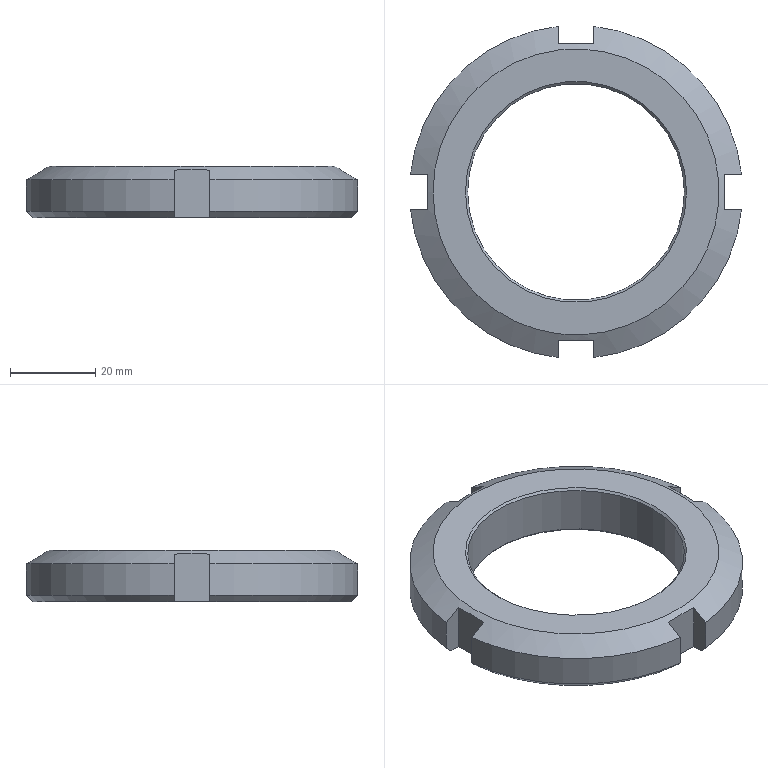Part | NX | features INSTANCE 4, CHAMFER 2, DATUM_CSYS 2, SKETCH 2, CIRCULAR_ISET 1, EXTRUDE 1, FSET 1, LINE 1, META 1, SWP104 1, SYMBOLIC_THREAD 1, THREADS 1, TRANSFORM_ISET 1 | 1 solid | 26 faces | box 77.551 x 77.551 x 12 mm | volume 29319 mm3 | plane 14 | cone 7 | cylinder 5 | commonest cylinder face diameters 78 x4 50.782 x1
STEP:
#1=CARTESIAN_POINT('',(-38.775,-4.18,1.5));
#2=VERTEX_POINT('',#1);
#3=CARTESIAN_POINT('',(-4.18,-38.775,1.5));
#4=VERTEX_POINT('',#3);
#5=CARTESIAN_POINT('',(0.,0.,1.5));
#6=DIRECTION('',(0.,0.,1.));
#7=DIRECTION('',(1.,0.,0.));
#8=AXIS2_PLACEMENT_3D('',#5,#6,#7);
#9=CIRCLE('',#8,39.);
#10=EDGE_CURVE('',#2,#4,#9,.T.);
#11=ORIENTED_EDGE('',*,*,#10,.T.);
#12=CARTESIAN_POINT('',(-4.18,-38.775,8.825));
#13=VERTEX_POINT('',#12);
#14=CARTESIAN_POINT('',(-4.18,-38.775,0.));
#15=DIRECTION('',(0.,0.,-1.));
#16=VECTOR('',#15,1000.);
#17=LINE('',#14,#16);
#18=EDGE_CURVE('',#4,#13,#17,.F.);
#19=ORIENTED_EDGE('',*,*,#18,.T.);
#20=CARTESIAN_POINT('',(-38.775,-4.18,8.825));
#21=VERTEX_POINT('',#20);
#22=CARTESIAN_POINT('',(0.,0.,8.825));
#23=DIRECTION('',(0.,0.,-1.));
#24=DIRECTION('',(-1.,0.,0.));
#25=AXIS2_PLACEMENT_3D('',#22,#23,#24);
#26=CIRCLE('',#25,39.);
#27=EDGE_CURVE('',#13,#21,#26,.T.);
#28=ORIENTED_EDGE('',*,*,#27,.T.);
#29=CARTESIAN_POINT('',(-38.775,-4.18,0.));
#30=DIRECTION('',(0.,0.,-1.));
#31=VECTOR('',#30,1000.);
#32=LINE('',#29,#31);
#33=EDGE_CURVE('',#21,#2,#32,.T.);
#34=ORIENTED_EDGE('',*,*,#33,.T.);
#35=EDGE_LOOP('',(#11,#19,#28,#34));
#36=FACE_BOUND('',#35,.T.);
#37=CARTESIAN_POINT('',(0.,0.,0.));
#38=DIRECTION('',(0.,0.,-1.));
#39=DIRECTION('',(-1.,0.,0.));
#40=AXIS2_PLACEMENT_3D('',#37,#38,#39);
#41=CYLINDRICAL_SURFACE('',#40,39.);
#42=ADVANCED_FACE('',(#36),#41,.T.);
#43=CARTESIAN_POINT('',(-4.18,-37.266,0.));
#44=VERTEX_POINT('',#43);
#45=CARTESIAN_POINT('',(-4.18,-38.775,1.5));
#46=CARTESIAN_POINT('',(-4.18,-38.272,0.9999));
#47=CARTESIAN_POINT('',(-4.18,-37.769,0.4999));
#48=CARTESIAN_POINT('',(-4.18,-37.266,0.));
#49=B_SPLINE_CURVE_WITH_KNOTS('',3,(#45,#46,#47,#48),.UNSPECIFIED.,.F.,.F.,(4,4),(0.008129,0.01026),.UNSPECIFIED.);
#50=EDGE_CURVE('',#4,#44,#49,.T.);
#51=ORIENTED_EDGE('',*,*,#50,.F.);
#52=ORIENTED_EDGE('',*,*,#10,.F.);
#53=CARTESIAN_POINT('',(-37.266,-4.18,0.));
#54=VERTEX_POINT('',#53);
#55=CARTESIAN_POINT('',(-37.266,-4.18,0.));
#56=CARTESIAN_POINT('',(-37.769,-4.18,0.4999));
#57=CARTESIAN_POINT('',(-38.272,-4.18,0.9999));
#58=CARTESIAN_POINT('',(-38.775,-4.18,1.5));
#59=B_SPLINE_CURVE_WITH_KNOTS('',3,(#55,#56,#57,#58),.UNSPECIFIED.,.F.,.F.,(4,4),(0.007494,0.009622),.UNSPECIFIED.);
#60=EDGE_CURVE('',#54,#2,#59,.T.);
#61=ORIENTED_EDGE('',*,*,#60,.F.);
#62=CARTESIAN_POINT('',(0.,0.,0.));
#63=DIRECTION('',(0.,0.,1.));
#64=DIRECTION('',(1.,0.,0.));
#65=AXIS2_PLACEMENT_3D('',#62,#63,#64);
#66=CIRCLE('',#65,37.5);
#67=EDGE_CURVE('',#44,#54,#66,.F.);
#68=ORIENTED_EDGE('',*,*,#67,.F.);
#69=EDGE_LOOP('',(#51,#52,#61,#68));
#70=FACE_BOUND('',#69,.T.);
#71=CARTESIAN_POINT('',(0.,0.,0.));
#72=DIRECTION('',(0.,0.,1.));
#73=DIRECTION('',(1.,0.,0.));
#74=AXIS2_PLACEMENT_3D('',#71,#72,#73);
#75=CONICAL_SURFACE('',#74,37.5,0.7854);
#76=ADVANCED_FACE('',(#70),#75,.T.);
#77=CARTESIAN_POINT('',(-4.18,38.775,1.5));
#78=VERTEX_POINT('',#77);
#79=CARTESIAN_POINT('',(-38.775,4.18,1.5));
#80=VERTEX_POINT('',#79);
#81=CARTESIAN_POINT('',(0.,0.,1.5));
#82=DIRECTION('',(0.,0.,1.));
#83=DIRECTION('',(1.,0.,0.));
#84=AXIS2_PLACEMENT_3D('',#81,#82,#83);
#85=CIRCLE('',#84,39.);
#86=EDGE_CURVE('',#78,#80,#85,.T.);
#87=ORIENTED_EDGE('',*,*,#86,.T.);
#88=CARTESIAN_POINT('',(-38.775,4.18,8.825));
#89=VERTEX_POINT('',#88);
#90=CARTESIAN_POINT('',(-38.775,4.18,0.));
#91=DIRECTION('',(0.,0.,-1.));
#92=VECTOR('',#91,1000.);
#93=LINE('',#90,#92);
#94=EDGE_CURVE('',#80,#89,#93,.F.);
#95=ORIENTED_EDGE('',*,*,#94,.T.);
#96=CARTESIAN_POINT('',(-4.18,38.775,8.825));
#97=VERTEX_POINT('',#96);
#98=CARTESIAN_POINT('',(0.,0.,8.825));
#99=DIRECTION('',(0.,0.,-1.));
#100=DIRECTION('',(-1.,0.,0.));
#101=AXIS2_PLACEMENT_3D('',#98,#99,#100);
#102=CIRCLE('',#101,39.);
#103=EDGE_CURVE('',#89,#97,#102,.T.);
#104=ORIENTED_EDGE('',*,*,#103,.T.);
#105=CARTESIAN_POINT('',(-4.18,38.775,0.));
#106=DIRECTION('',(0.,0.,-1.));
#107=VECTOR('',#106,1000.);
#108=LINE('',#105,#107);
#109=EDGE_CURVE('',#97,#78,#108,.T.);
#110=ORIENTED_EDGE('',*,*,#109,.T.);
#111=EDGE_LOOP('',(#87,#95,#104,#110));
#112=FACE_BOUND('',#111,.T.);
#113=CARTESIAN_POINT('',(0.,0.,0.));
#114=DIRECTION('',(0.,0.,-1.));
#115=DIRECTION('',(-1.,0.,0.));
#116=AXIS2_PLACEMENT_3D('',#113,#114,#115);
#117=CYLINDRICAL_SURFACE('',#116,39.);
#118=ADVANCED_FACE('',(#112),#117,.T.);
#119=CARTESIAN_POINT('',(-37.266,4.18,0.));
#120=VERTEX_POINT('',#119);
#121=CARTESIAN_POINT('',(-38.775,4.18,1.5));
#122=CARTESIAN_POINT('',(-38.272,4.18,0.9999));
#123=CARTESIAN_POINT('',(-37.769,4.18,0.4999));
#124=CARTESIAN_POINT('',(-37.266,4.18,0.));
#125=B_SPLINE_CURVE_WITH_KNOTS('',3,(#121,#122,#123,#124),.UNSPECIFIED.,.F.,.F.,(4,4),(0.008129,0.01026),.UNSPECIFIED.);
#126=EDGE_CURVE('',#80,#120,#125,.T.);
#127=ORIENTED_EDGE('',*,*,#126,.F.);
#128=ORIENTED_EDGE('',*,*,#86,.F.);
#129=CARTESIAN_POINT('',(-4.18,37.266,0.));
#130=VERTEX_POINT('',#129);
#131=CARTESIAN_POINT('',(-4.18,37.266,0.));
#132=CARTESIAN_POINT('',(-4.18,37.769,0.4999));
#133=CARTESIAN_POINT('',(-4.18,38.272,0.9999));
#134=CARTESIAN_POINT('',(-4.18,38.775,1.5));
#135=B_SPLINE_CURVE_WITH_KNOTS('',3,(#131,#132,#133,#134),.UNSPECIFIED.,.F.,.F.,(4,4),(0.008247,0.01038),.UNSPECIFIED.);
#136=EDGE_CURVE('',#130,#78,#135,.T.);
#137=ORIENTED_EDGE('',*,*,#136,.F.);
#138=CARTESIAN_POINT('',(0.,0.,0.));
#139=DIRECTION('',(0.,0.,1.));
#140=DIRECTION('',(1.,0.,0.));
#141=AXIS2_PLACEMENT_3D('',#138,#139,#140);
#142=CIRCLE('',#141,37.5);
#143=EDGE_CURVE('',#120,#130,#142,.F.);
#144=ORIENTED_EDGE('',*,*,#143,.F.);
#145=EDGE_LOOP('',(#127,#128,#137,#144));
#146=FACE_BOUND('',#145,.T.);
#147=CARTESIAN_POINT('',(0.,0.,0.));
#148=DIRECTION('',(0.,0.,1.));
#149=DIRECTION('',(1.,0.,0.));
#150=AXIS2_PLACEMENT_3D('',#147,#148,#149);
#151=CONICAL_SURFACE('',#150,37.5,0.7854);
#152=ADVANCED_FACE('',(#146),#151,.T.);
#153=CARTESIAN_POINT('',(38.775,4.18,1.5));
#154=VERTEX_POINT('',#153);
#155=CARTESIAN_POINT('',(4.18,38.775,1.5));
#156=VERTEX_POINT('',#155);
#157=CARTESIAN_POINT('',(0.,0.,1.5));
#158=DIRECTION('',(0.,0.,1.));
#159=DIRECTION('',(1.,0.,0.));
#160=AXIS2_PLACEMENT_3D('',#157,#158,#159);
#161=CIRCLE('',#160,39.);
#162=EDGE_CURVE('',#154,#156,#161,.T.);
#163=ORIENTED_EDGE('',*,*,#162,.T.);
#164=CARTESIAN_POINT('',(4.18,38.775,8.825));
#165=VERTEX_POINT('',#164);
#166=CARTESIAN_POINT('',(4.18,38.775,0.));
#167=DIRECTION('',(0.,0.,-1.));
#168=VECTOR('',#167,1000.);
#169=LINE('',#166,#168);
#170=EDGE_CURVE('',#156,#165,#169,.F.);
#171=ORIENTED_EDGE('',*,*,#170,.T.);
#172=CARTESIAN_POINT('',(38.775,4.18,8.825));
#173=VERTEX_POINT('',#172);
#174=CARTESIAN_POINT('',(0.,0.,8.825));
#175=DIRECTION('',(0.,0.,-1.));
#176=DIRECTION('',(-1.,0.,0.));
#177=AXIS2_PLACEMENT_3D('',#174,#175,#176);
#178=CIRCLE('',#177,39.);
#179=EDGE_CURVE('',#165,#173,#178,.T.);
#180=ORIENTED_EDGE('',*,*,#179,.T.);
#181=CARTESIAN_POINT('',(38.775,4.18,0.));
#182=DIRECTION('',(0.,0.,-1.));
#183=VECTOR('',#182,1000.);
#184=LINE('',#181,#183);
#185=EDGE_CURVE('',#173,#154,#184,.T.);
#186=ORIENTED_EDGE('',*,*,#185,.T.);
#187=EDGE_LOOP('',(#163,#171,#180,#186));
#188=FACE_BOUND('',#187,.T.);
#189=CARTESIAN_POINT('',(0.,0.,0.));
#190=DIRECTION('',(0.,0.,-1.));
#191=DIRECTION('',(-1.,0.,0.));
#192=AXIS2_PLACEMENT_3D('',#189,#190,#191);
#193=CYLINDRICAL_SURFACE('',#192,39.);
#194=ADVANCED_FACE('',(#188),#193,.T.);
#195=CARTESIAN_POINT('',(4.18,37.266,0.));
#196=VERTEX_POINT('',#195);
#197=CARTESIAN_POINT('',(4.18,38.775,1.5));
#198=CARTESIAN_POINT('',(4.18,38.272,0.9999));
#199=CARTESIAN_POINT('',(4.18,37.769,0.4999));
#200=CARTESIAN_POINT('',(4.18,37.266,0.));
#201=B_SPLINE_CURVE_WITH_KNOTS('',3,(#197,#198,#199,#200),.UNSPECIFIED.,.F.,.F.,(4,4),(0.007376,0.009503),.UNSPECIFIED.);
#202=EDGE_CURVE('',#156,#196,#201,.T.);
#203=ORIENTED_EDGE('',*,*,#202,.F.);
#204=ORIENTED_EDGE('',*,*,#162,.F.);
#205=CARTESIAN_POINT('',(37.266,4.18,0.));
#206=VERTEX_POINT('',#205);
#207=CARTESIAN_POINT('',(37.266,4.18,0.));
#208=CARTESIAN_POINT('',(37.769,4.18,0.4999));
#209=CARTESIAN_POINT('',(38.272,4.18,0.9999));
#210=CARTESIAN_POINT('',(38.775,4.18,1.5));
#211=B_SPLINE_CURVE_WITH_KNOTS('',3,(#207,#208,#209,#210),.UNSPECIFIED.,.F.,.F.,(4,4),(0.008247,0.01038),.UNSPECIFIED.);
#212=EDGE_CURVE('',#206,#154,#211,.T.);
#213=ORIENTED_EDGE('',*,*,#212,.F.);
#214=CARTESIAN_POINT('',(0.,0.,0.));
#215=DIRECTION('',(0.,0.,1.));
#216=DIRECTION('',(1.,0.,0.));
#217=AXIS2_PLACEMENT_3D('',#214,#215,#216);
#218=CIRCLE('',#217,37.5);
#219=EDGE_CURVE('',#196,#206,#218,.F.);
#220=ORIENTED_EDGE('',*,*,#219,.F.);
#221=EDGE_LOOP('',(#203,#204,#213,#220));
#222=FACE_BOUND('',#221,.T.);
#223=CARTESIAN_POINT('',(0.,0.,0.));
#224=DIRECTION('',(0.,0.,1.));
#225=DIRECTION('',(1.,0.,0.));
#226=AXIS2_PLACEMENT_3D('',#223,#224,#225);
#227=CONICAL_SURFACE('',#226,37.5,0.7854);
#228=ADVANCED_FACE('',(#222),#227,.T.);
#229=CARTESIAN_POINT('',(25.891,0.,0.));
#230=VERTEX_POINT('',#229);
#231=CARTESIAN_POINT('',(0.,0.,0.));
#232=DIRECTION('',(0.,0.,1.));
#233=DIRECTION('',(1.,0.,0.));
#234=AXIS2_PLACEMENT_3D('',#231,#232,#233);
#235=CIRCLE('',#234,25.891);
#236=EDGE_CURVE('',#230,#230,#235,.T.);
#237=ORIENTED_EDGE('',*,*,#236,.T.);
#238=EDGE_LOOP('',(#237));
#239=FACE_BOUND('',#238,.T.);
#240=CARTESIAN_POINT('',(-4.18,-34.75,0.));
#241=VERTEX_POINT('',#240);
#242=CARTESIAN_POINT('',(4.18,-34.75,0.));
#243=VERTEX_POINT('',#242);
#244=CARTESIAN_POINT('',(-4.18,-34.75,0.));
#245=DIRECTION('',(1.,0.,0.));
#246=VECTOR('',#245,1000.);
#247=LINE('',#244,#246);
#248=EDGE_CURVE('',#241,#243,#247,.T.);
#249=ORIENTED_EDGE('',*,*,#248,.F.);
#250=CARTESIAN_POINT('',(-4.18,-73.75,0.));
#251=DIRECTION('',(0.,1.,0.));
#252=VECTOR('',#251,1000.);
#253=LINE('',#250,#252);
#254=EDGE_CURVE('',#44,#241,#253,.T.);
#255=ORIENTED_EDGE('',*,*,#254,.F.);
#256=ORIENTED_EDGE('',*,*,#67,.T.);
#257=CARTESIAN_POINT('',(-34.75,-4.18,0.));
#258=VERTEX_POINT('',#257);
#259=CARTESIAN_POINT('',(-34.75,-4.18,0.));
#260=DIRECTION('',(-1.,0.,0.));
#261=VECTOR('',#260,1000.);
#262=LINE('',#259,#261);
#263=EDGE_CURVE('',#258,#54,#262,.T.);
#264=ORIENTED_EDGE('',*,*,#263,.F.);
#265=CARTESIAN_POINT('',(-34.75,4.18,0.));
#266=VERTEX_POINT('',#265);
#267=CARTESIAN_POINT('',(-34.75,4.18,0.));
#268=DIRECTION('',(0.,-1.,0.));
#269=VECTOR('',#268,1000.);
#270=LINE('',#267,#269);
#271=EDGE_CURVE('',#266,#258,#270,.T.);
#272=ORIENTED_EDGE('',*,*,#271,.F.);
#273=CARTESIAN_POINT('',(-73.75,4.18,0.));
#274=DIRECTION('',(1.,0.,0.));
#275=VECTOR('',#274,1000.);
#276=LINE('',#273,#275);
#277=EDGE_CURVE('',#120,#266,#276,.T.);
#278=ORIENTED_EDGE('',*,*,#277,.F.);
#279=ORIENTED_EDGE('',*,*,#143,.T.);
#280=CARTESIAN_POINT('',(-4.18,34.75,0.));
#281=VERTEX_POINT('',#280);
#282=CARTESIAN_POINT('',(-4.18,34.75,0.));
#283=DIRECTION('',(0.,1.,0.));
#284=VECTOR('',#283,1000.);
#285=LINE('',#282,#284);
#286=EDGE_CURVE('',#281,#130,#285,.T.);
#287=ORIENTED_EDGE('',*,*,#286,.F.);
#288=CARTESIAN_POINT('',(4.18,34.75,0.));
#289=VERTEX_POINT('',#288);
#290=CARTESIAN_POINT('',(4.18,34.75,0.));
#291=DIRECTION('',(-1.,0.,0.));
#292=VECTOR('',#291,1000.);
#293=LINE('',#290,#292);
#294=EDGE_CURVE('',#289,#281,#293,.T.);
#295=ORIENTED_EDGE('',*,*,#294,.F.);
#296=CARTESIAN_POINT('',(4.18,73.75,0.));
#297=DIRECTION('',(0.,-1.,0.));
#298=VECTOR('',#297,1000.);
#299=LINE('',#296,#298);
#300=EDGE_CURVE('',#196,#289,#299,.T.);
#301=ORIENTED_EDGE('',*,*,#300,.F.);
#302=ORIENTED_EDGE('',*,*,#219,.T.);
#303=CARTESIAN_POINT('',(34.75,4.18,0.));
#304=VERTEX_POINT('',#303);
#305=CARTESIAN_POINT('',(34.75,4.18,0.));
#306=DIRECTION('',(1.,0.,0.));
#307=VECTOR('',#306,1000.);
#308=LINE('',#305,#307);
#309=EDGE_CURVE('',#304,#206,#308,.T.);
#310=ORIENTED_EDGE('',*,*,#309,.F.);
#311=CARTESIAN_POINT('',(34.75,-4.18,0.));
#312=VERTEX_POINT('',#311);
#313=CARTESIAN_POINT('',(34.75,-4.18,0.));
#314=DIRECTION('',(0.,1.,0.));
#315=VECTOR('',#314,1000.);
#316=LINE('',#313,#315);
#317=EDGE_CURVE('',#312,#304,#316,.T.);
#318=ORIENTED_EDGE('',*,*,#317,.F.);
#319=CARTESIAN_POINT('',(37.266,-4.18,0.));
#320=VERTEX_POINT('',#319);
#321=CARTESIAN_POINT('',(73.75,-4.18,0.));
#322=DIRECTION('',(-1.,0.,0.));
#323=VECTOR('',#322,1000.);
#324=LINE('',#321,#323);
#325=EDGE_CURVE('',#320,#312,#324,.T.);
#326=ORIENTED_EDGE('',*,*,#325,.F.);
#327=CARTESIAN_POINT('',(4.18,-37.266,0.));
#328=VERTEX_POINT('',#327);
#329=CARTESIAN_POINT('',(0.,0.,0.));
#330=DIRECTION('',(0.,0.,1.));
#331=DIRECTION('',(1.,0.,0.));
#332=AXIS2_PLACEMENT_3D('',#329,#330,#331);
#333=CIRCLE('',#332,37.5);
#334=EDGE_CURVE('',#320,#328,#333,.F.);
#335=ORIENTED_EDGE('',*,*,#334,.T.);
#336=CARTESIAN_POINT('',(4.18,-34.75,0.));
#337=DIRECTION('',(0.,-1.,0.));
#338=VECTOR('',#337,1000.);
#339=LINE('',#336,#338);
#340=EDGE_CURVE('',#243,#328,#339,.T.);
#341=ORIENTED_EDGE('',*,*,#340,.F.);
#342=EDGE_LOOP('',(#249,#255,#256,#264,#272,#278,#279,#287,#295,#301,#302,#310,#318,#326,#335,#341));
#343=FACE_BOUND('',#342,.T.);
#344=CARTESIAN_POINT('',(39.,0.,0.));
#345=DIRECTION('',(0.,0.,1.));
#346=DIRECTION('',(1.,0.,0.));
#347=AXIS2_PLACEMENT_3D('',#344,#345,#346);
#348=PLANE('',#347);
#349=ADVANCED_FACE('',(#239,#343),#348,.F.);
#350=ORIENTED_EDGE('',*,*,#27,.F.);
#351=CARTESIAN_POINT('',(-4.18,-34.75,11.134));
#352=VERTEX_POINT('',#351);
#353=CARTESIAN_POINT('',(-4.18,-38.775,8.825));
#354=CARTESIAN_POINT('',(-4.18,-37.434,9.595));
#355=CARTESIAN_POINT('',(-4.18,-36.092,10.364));
#356=CARTESIAN_POINT('',(-4.18,-34.75,11.134));
#357=B_SPLINE_CURVE_WITH_KNOTS('',3,(#353,#354,#355,#356),.UNSPECIFIED.,.F.,.F.,(4,4),(0.009426,0.01407),.UNSPECIFIED.);
#358=EDGE_CURVE('',#13,#352,#357,.T.);
#359=ORIENTED_EDGE('',*,*,#358,.T.);
#360=CARTESIAN_POINT('',(4.18,-34.75,11.134));
#361=VERTEX_POINT('',#360);
#362=CARTESIAN_POINT('',(-4.18,-34.75,11.134));
#363=CARTESIAN_POINT('',(-1.387,-34.75,11.326));
#364=CARTESIAN_POINT('',(1.41,-34.75,11.325));
#365=CARTESIAN_POINT('',(4.18,-34.75,11.134));
#366=B_SPLINE_CURVE_WITH_KNOTS('',3,(#362,#363,#364,#365),.UNSPECIFIED.,.F.,.F.,(4,4),(0.01696,0.02531),.UNSPECIFIED.);
#367=EDGE_CURVE('',#352,#361,#366,.T.);
#368=ORIENTED_EDGE('',*,*,#367,.T.);
#369=CARTESIAN_POINT('',(4.18,-38.775,8.825));
#370=VERTEX_POINT('',#369);
#371=CARTESIAN_POINT('',(4.18,-34.75,11.134));
#372=CARTESIAN_POINT('',(4.18,-36.092,10.364));
#373=CARTESIAN_POINT('',(4.18,-37.434,9.595));
#374=CARTESIAN_POINT('',(4.18,-38.775,8.825));
#375=B_SPLINE_CURVE_WITH_KNOTS('',3,(#371,#372,#373,#374),.UNSPECIFIED.,.F.,.F.,(4,4),(0.006108,0.01075),.UNSPECIFIED.);
#376=EDGE_CURVE('',#361,#370,#375,.T.);
#377=ORIENTED_EDGE('',*,*,#376,.T.);
#378=CARTESIAN_POINT('',(38.775,-4.18,8.825));
#379=VERTEX_POINT('',#378);
#380=CARTESIAN_POINT('',(0.,0.,8.825));
#381=DIRECTION('',(0.,0.,-1.));
#382=DIRECTION('',(-1.,0.,0.));
#383=AXIS2_PLACEMENT_3D('',#380,#381,#382);
#384=CIRCLE('',#383,39.);
#385=EDGE_CURVE('',#379,#370,#384,.T.);
#386=ORIENTED_EDGE('',*,*,#385,.F.);
#387=CARTESIAN_POINT('',(34.75,-4.18,11.134));
#388=VERTEX_POINT('',#387);
#389=CARTESIAN_POINT('',(38.775,-4.18,8.825));
#390=CARTESIAN_POINT('',(37.434,-4.18,9.595));
#391=CARTESIAN_POINT('',(36.092,-4.18,10.364));
#392=CARTESIAN_POINT('',(34.75,-4.18,11.134));
#393=B_SPLINE_CURVE_WITH_KNOTS('',3,(#389,#390,#391,#392),.UNSPECIFIED.,.F.,.F.,(4,4),(0.007583,0.01222),.UNSPECIFIED.);
#394=EDGE_CURVE('',#379,#388,#393,.T.);
#395=ORIENTED_EDGE('',*,*,#394,.T.);
#396=CARTESIAN_POINT('',(34.75,4.18,11.134));
#397=VERTEX_POINT('',#396);
#398=CARTESIAN_POINT('',(34.75,-4.18,11.134));
#399=CARTESIAN_POINT('',(34.75,-1.387,11.326));
#400=CARTESIAN_POINT('',(34.75,1.41,11.325));
#401=CARTESIAN_POINT('',(34.75,4.18,11.134));
#402=B_SPLINE_CURVE_WITH_KNOTS('',3,(#398,#399,#400,#401),.UNSPECIFIED.,.F.,.F.,(4,4),(0.01696,0.02531),.UNSPECIFIED.);
#403=EDGE_CURVE('',#388,#397,#402,.T.);
#404=ORIENTED_EDGE('',*,*,#403,.T.);
#405=CARTESIAN_POINT('',(34.75,4.18,11.134));
#406=CARTESIAN_POINT('',(36.092,4.18,10.364));
#407=CARTESIAN_POINT('',(37.434,4.18,9.595));
#408=CARTESIAN_POINT('',(38.775,4.18,8.825));
#409=B_SPLINE_CURVE_WITH_KNOTS('',3,(#405,#406,#407,#408),.UNSPECIFIED.,.F.,.F.,(4,4),(0.007951,0.01259),.UNSPECIFIED.);
#410=EDGE_CURVE('',#397,#173,#409,.T.);
#411=ORIENTED_EDGE('',*,*,#410,.T.);
#412=ORIENTED_EDGE('',*,*,#179,.F.);
#413=CARTESIAN_POINT('',(4.18,34.75,11.134));
#414=VERTEX_POINT('',#413);
#415=CARTESIAN_POINT('',(4.18,38.775,8.825));
#416=CARTESIAN_POINT('',(4.18,37.434,9.595));
#417=CARTESIAN_POINT('',(4.18,36.092,10.364));
#418=CARTESIAN_POINT('',(4.18,34.75,11.134));
#419=B_SPLINE_CURVE_WITH_KNOTS('',3,(#415,#416,#417,#418),.UNSPECIFIED.,.F.,.F.,(4,4),(0.007583,0.01222),.UNSPECIFIED.);
#420=EDGE_CURVE('',#165,#414,#419,.T.);
#421=ORIENTED_EDGE('',*,*,#420,.T.);
#422=CARTESIAN_POINT('',(-4.18,34.75,11.134));
#423=VERTEX_POINT('',#422);
#424=CARTESIAN_POINT('',(4.18,34.75,11.134));
#425=CARTESIAN_POINT('',(1.41,34.75,11.325));
#426=CARTESIAN_POINT('',(-1.387,34.75,11.326));
#427=CARTESIAN_POINT('',(-4.18,34.75,11.134));
#428=B_SPLINE_CURVE_WITH_KNOTS('',3,(#424,#425,#426,#427),.UNSPECIFIED.,.F.,.F.,(4,4),(0.01067,0.01899),.UNSPECIFIED.);
#429=EDGE_CURVE('',#414,#423,#428,.T.);
#430=ORIENTED_EDGE('',*,*,#429,.T.);
#431=CARTESIAN_POINT('',(-4.18,34.75,11.134));
#432=CARTESIAN_POINT('',(-4.18,36.092,10.364));
#433=CARTESIAN_POINT('',(-4.18,37.434,9.595));
#434=CARTESIAN_POINT('',(-4.18,38.775,8.825));
#435=B_SPLINE_CURVE_WITH_KNOTS('',3,(#431,#432,#433,#434),.UNSPECIFIED.,.F.,.F.,(4,4),(0.007951,0.01259),.UNSPECIFIED.);
#436=EDGE_CURVE('',#423,#97,#435,.T.);
#437=ORIENTED_EDGE('',*,*,#436,.T.);
#438=ORIENTED_EDGE('',*,*,#103,.F.);
#439=CARTESIAN_POINT('',(-34.75,4.18,11.134));
#440=VERTEX_POINT('',#439);
#441=CARTESIAN_POINT('',(-38.775,4.18,8.825));
#442=CARTESIAN_POINT('',(-37.434,4.18,9.595));
#443=CARTESIAN_POINT('',(-36.092,4.18,10.364));
#444=CARTESIAN_POINT('',(-34.75,4.18,11.134));
#445=B_SPLINE_CURVE_WITH_KNOTS('',3,(#441,#442,#443,#444),.UNSPECIFIED.,.F.,.F.,(4,4),(0.009426,0.01407),.UNSPECIFIED.);
#446=EDGE_CURVE('',#89,#440,#445,.T.);
#447=ORIENTED_EDGE('',*,*,#446,.T.);
#448=CARTESIAN_POINT('',(-34.75,-4.18,11.134));
#449=VERTEX_POINT('',#448);
#450=CARTESIAN_POINT('',(-34.75,4.18,11.134));
#451=CARTESIAN_POINT('',(-34.75,1.41,11.325));
#452=CARTESIAN_POINT('',(-34.75,-1.387,11.326));
#453=CARTESIAN_POINT('',(-34.75,-4.18,11.134));
#454=B_SPLINE_CURVE_WITH_KNOTS('',3,(#450,#451,#452,#453),.UNSPECIFIED.,.F.,.F.,(4,4),(0.01067,0.01899),.UNSPECIFIED.);
#455=EDGE_CURVE('',#440,#449,#454,.T.);
#456=ORIENTED_EDGE('',*,*,#455,.T.);
#457=CARTESIAN_POINT('',(-34.75,-4.18,11.134));
#458=CARTESIAN_POINT('',(-36.092,-4.18,10.364));
#459=CARTESIAN_POINT('',(-37.434,-4.18,9.595));
#460=CARTESIAN_POINT('',(-38.775,-4.18,8.825));
#461=B_SPLINE_CURVE_WITH_KNOTS('',3,(#457,#458,#459,#460),.UNSPECIFIED.,.F.,.F.,(4,4),(0.006108,0.01075),.UNSPECIFIED.);
#462=EDGE_CURVE('',#449,#21,#461,.T.);
#463=ORIENTED_EDGE('',*,*,#462,.T.);
#464=EDGE_LOOP('',(#350,#359,#368,#377,#386,#395,#404,#411,#412,#421,#430,#437,#438,#447,#456,#463));
#465=FACE_BOUND('',#464,.T.);
#466=CARTESIAN_POINT('',(-33.5,0.,12.));
#467=VERTEX_POINT('',#466);
#468=CARTESIAN_POINT('',(0.,0.,12.));
#469=DIRECTION('',(0.,0.,-1.));
#470=DIRECTION('',(-1.,0.,0.));
#471=AXIS2_PLACEMENT_3D('',#468,#469,#470);
#472=CIRCLE('',#471,33.5);
#473=EDGE_CURVE('',#467,#467,#472,.T.);
#474=ORIENTED_EDGE('',*,*,#473,.T.);
#475=EDGE_LOOP('',(#474));
#476=FACE_BOUND('',#475,.T.);
#477=CARTESIAN_POINT('',(0.,0.,12.));
#478=DIRECTION('',(0.,0.,-1.));
#479=DIRECTION('',(-1.,0.,0.));
#480=AXIS2_PLACEMENT_3D('',#477,#478,#479);
#481=CONICAL_SURFACE('',#480,33.5,1.047);
#482=ADVANCED_FACE('',(#465,#476),#481,.T.);
#483=ORIENTED_EDGE('',*,*,#385,.T.);
#484=CARTESIAN_POINT('',(4.18,-38.775,1.5));
#485=VERTEX_POINT('',#484);
#486=CARTESIAN_POINT('',(4.18,-38.775,0.));
#487=DIRECTION('',(0.,0.,-1.));
#488=VECTOR('',#487,1000.);
#489=LINE('',#486,#488);
#490=EDGE_CURVE('',#370,#485,#489,.T.);
#491=ORIENTED_EDGE('',*,*,#490,.T.);
#492=CARTESIAN_POINT('',(38.775,-4.18,1.5));
#493=VERTEX_POINT('',#492);
#494=CARTESIAN_POINT('',(0.,0.,1.5));
#495=DIRECTION('',(0.,0.,1.));
#496=DIRECTION('',(1.,0.,0.));
#497=AXIS2_PLACEMENT_3D('',#494,#495,#496);
#498=CIRCLE('',#497,39.);
#499=EDGE_CURVE('',#485,#493,#498,.T.);
#500=ORIENTED_EDGE('',*,*,#499,.T.);
#501=CARTESIAN_POINT('',(38.775,-4.18,0.));
#502=DIRECTION('',(0.,0.,-1.));
#503=VECTOR('',#502,1000.);
#504=LINE('',#501,#503);
#505=EDGE_CURVE('',#493,#379,#504,.F.);
#506=ORIENTED_EDGE('',*,*,#505,.T.);
#507=EDGE_LOOP('',(#483,#491,#500,#506));
#508=FACE_BOUND('',#507,.T.);
#509=CARTESIAN_POINT('',(0.,0.,0.));
#510=DIRECTION('',(0.,0.,-1.));
#511=DIRECTION('',(-1.,0.,0.));
#512=AXIS2_PLACEMENT_3D('',#509,#510,#511);
#513=CYLINDRICAL_SURFACE('',#512,39.);
#514=ADVANCED_FACE('',(#508),#513,.T.);
#515=CARTESIAN_POINT('',(25.391,0.,0.5));
#516=VERTEX_POINT('',#515);
#517=CARTESIAN_POINT('',(0.,0.,0.5));
#518=DIRECTION('',(0.,0.,1.));
#519=DIRECTION('',(1.,0.,0.));
#520=AXIS2_PLACEMENT_3D('',#517,#518,#519);
#521=CIRCLE('',#520,25.391);
#522=EDGE_CURVE('',#516,#516,#521,.F.);
#523=ORIENTED_EDGE('',*,*,#522,.T.);
#524=EDGE_LOOP('',(#523));
#525=FACE_BOUND('',#524,.T.);
#526=CARTESIAN_POINT('',(-25.391,0.,11.5));
#527=VERTEX_POINT('',#526);
#528=CARTESIAN_POINT('',(0.,0.,11.5));
#529=DIRECTION('',(0.,0.,-1.));
#530=DIRECTION('',(-1.,0.,0.));
#531=AXIS2_PLACEMENT_3D('',#528,#529,#530);
#532=CIRCLE('',#531,25.391);
#533=EDGE_CURVE('',#527,#527,#532,.F.);
#534=ORIENTED_EDGE('',*,*,#533,.T.);
#535=EDGE_LOOP('',(#534));
#536=FACE_BOUND('',#535,.T.);
#537=CARTESIAN_POINT('',(0.,0.,0.));
#538=DIRECTION('',(0.,0.,-1.));
#539=DIRECTION('',(-1.,0.,0.));
#540=AXIS2_PLACEMENT_3D('',#537,#538,#539);
#541=CYLINDRICAL_SURFACE('',#540,25.391);
#542=ADVANCED_FACE('',(#525,#536),#541,.F.);
#543=CARTESIAN_POINT('',(-25.891,0.,12.));
#544=VERTEX_POINT('',#543);
#545=CARTESIAN_POINT('',(0.,0.,12.));
#546=DIRECTION('',(0.,0.,-1.));
#547=DIRECTION('',(-1.,0.,0.));
#548=AXIS2_PLACEMENT_3D('',#545,#546,#547);
#549=CIRCLE('',#548,25.891);
#550=EDGE_CURVE('',#544,#544,#549,.T.);
#551=ORIENTED_EDGE('',*,*,#550,.T.);
#552=EDGE_LOOP('',(#551));
#553=FACE_BOUND('',#552,.T.);
#554=ORIENTED_EDGE('',*,*,#473,.F.);
#555=EDGE_LOOP('',(#554));
#556=FACE_BOUND('',#555,.T.);
#557=CARTESIAN_POINT('',(25.391,0.,12.));
#558=DIRECTION('',(0.,0.,-1.));
#559=DIRECTION('',(-1.,0.,0.));
#560=AXIS2_PLACEMENT_3D('',#557,#558,#559);
#561=PLANE('',#560);
#562=ADVANCED_FACE('',(#553,#556),#561,.F.);
#563=CARTESIAN_POINT('',(4.18,-37.266,0.));
#564=CARTESIAN_POINT('',(4.18,-37.769,0.4999));
#565=CARTESIAN_POINT('',(4.18,-38.272,0.9999));
#566=CARTESIAN_POINT('',(4.18,-38.775,1.5));
#567=B_SPLINE_CURVE_WITH_KNOTS('',3,(#563,#564,#565,#566),.UNSPECIFIED.,.F.,.F.,(4,4),(0.007494,0.009622),.UNSPECIFIED.);
#568=EDGE_CURVE('',#328,#485,#567,.T.);
#569=ORIENTED_EDGE('',*,*,#568,.F.);
#570=ORIENTED_EDGE('',*,*,#334,.F.);
#571=CARTESIAN_POINT('',(38.775,-4.18,1.5));
#572=CARTESIAN_POINT('',(38.272,-4.18,0.9999));
#573=CARTESIAN_POINT('',(37.769,-4.18,0.4999));
#574=CARTESIAN_POINT('',(37.266,-4.18,0.));
#575=B_SPLINE_CURVE_WITH_KNOTS('',3,(#571,#572,#573,#574),.UNSPECIFIED.,.F.,.F.,(4,4),(0.007376,0.009503),.UNSPECIFIED.);
#576=EDGE_CURVE('',#493,#320,#575,.T.);
#577=ORIENTED_EDGE('',*,*,#576,.F.);
#578=ORIENTED_EDGE('',*,*,#499,.F.);
#579=EDGE_LOOP('',(#569,#570,#577,#578));
#580=FACE_BOUND('',#579,.T.);
#581=CARTESIAN_POINT('',(0.,0.,0.));
#582=DIRECTION('',(0.,0.,1.));
#583=DIRECTION('',(1.,0.,0.));
#584=AXIS2_PLACEMENT_3D('',#581,#582,#583);
#585=CONICAL_SURFACE('',#584,37.5,0.7854);
#586=ADVANCED_FACE('',(#580),#585,.T.);
#587=ORIENTED_EDGE('',*,*,#236,.F.);
#588=EDGE_LOOP('',(#587));
#589=FACE_BOUND('',#588,.T.);
#590=ORIENTED_EDGE('',*,*,#522,.F.);
#591=EDGE_LOOP('',(#590));
#592=FACE_BOUND('',#591,.T.);
#593=CARTESIAN_POINT('',(0.,0.,0.5));
#594=DIRECTION('',(0.,0.,-1.));
#595=DIRECTION('',(-1.,0.,0.));
#596=AXIS2_PLACEMENT_3D('',#593,#594,#595);
#597=CONICAL_SURFACE('',#596,25.391,0.7854);
#598=ADVANCED_FACE('',(#589,#592),#597,.F.);
#599=ORIENTED_EDGE('',*,*,#533,.F.);
#600=EDGE_LOOP('',(#599));
#601=FACE_BOUND('',#600,.T.);
#602=ORIENTED_EDGE('',*,*,#550,.F.);
#603=EDGE_LOOP('',(#602));
#604=FACE_BOUND('',#603,.T.);
#605=CARTESIAN_POINT('',(0.,0.,12.));
#606=DIRECTION('',(0.,0.,1.));
#607=DIRECTION('',(1.,0.,0.));
#608=AXIS2_PLACEMENT_3D('',#605,#606,#607);
#609=CONICAL_SURFACE('',#608,25.891,0.7854);
#610=ADVANCED_FACE('',(#601,#604),#609,.F.);
#611=CARTESIAN_POINT('',(34.75,-4.18,12.));
#612=DIRECTION('',(0.,0.,-1.));
#613=VECTOR('',#612,1000.);
#614=LINE('',#611,#613);
#615=EDGE_CURVE('',#388,#312,#614,.T.);
#616=ORIENTED_EDGE('',*,*,#615,.T.);
#617=ORIENTED_EDGE('',*,*,#317,.T.);
#618=CARTESIAN_POINT('',(34.75,4.18,12.));
#619=DIRECTION('',(0.,0.,-1.));
#620=VECTOR('',#619,1000.);
#621=LINE('',#618,#620);
#622=EDGE_CURVE('',#397,#304,#621,.T.);
#623=ORIENTED_EDGE('',*,*,#622,.F.);
#624=ORIENTED_EDGE('',*,*,#403,.F.);
#625=EDGE_LOOP('',(#616,#617,#623,#624));
#626=FACE_BOUND('',#625,.T.);
#627=CARTESIAN_POINT('',(34.75,-4.18,12.));
#628=DIRECTION('',(-1.,0.,0.));
#629=DIRECTION('',(0.,0.,1.));
#630=AXIS2_PLACEMENT_3D('',#627,#628,#629);
#631=PLANE('',#630);
#632=ADVANCED_FACE('',(#626),#631,.F.);
#633=ORIENTED_EDGE('',*,*,#505,.F.);
#634=ORIENTED_EDGE('',*,*,#576,.T.);
#635=ORIENTED_EDGE('',*,*,#325,.T.);
#636=ORIENTED_EDGE('',*,*,#615,.F.);
#637=ORIENTED_EDGE('',*,*,#394,.F.);
#638=EDGE_LOOP('',(#633,#634,#635,#636,#637));
#639=FACE_BOUND('',#638,.T.);
#640=CARTESIAN_POINT('',(73.75,-4.18,12.));
#641=DIRECTION('',(0.,-1.,0.));
#642=DIRECTION('',(1.,0.,0.));
#643=AXIS2_PLACEMENT_3D('',#640,#641,#642);
#644=PLANE('',#643);
#645=ADVANCED_FACE('',(#639),#644,.F.);
#646=ORIENTED_EDGE('',*,*,#622,.T.);
#647=ORIENTED_EDGE('',*,*,#309,.T.);
#648=ORIENTED_EDGE('',*,*,#212,.T.);
#649=ORIENTED_EDGE('',*,*,#185,.F.);
#650=ORIENTED_EDGE('',*,*,#410,.F.);
#651=EDGE_LOOP('',(#646,#647,#648,#649,#650));
#652=FACE_BOUND('',#651,.T.);
#653=CARTESIAN_POINT('',(34.75,4.18,12.));
#654=DIRECTION('',(0.,1.,0.));
#655=DIRECTION('',(-1.,0.,0.));
#656=AXIS2_PLACEMENT_3D('',#653,#654,#655);
#657=PLANE('',#656);
#658=ADVANCED_FACE('',(#652),#657,.F.);
#659=CARTESIAN_POINT('',(4.18,34.75,12.));
#660=DIRECTION('',(0.,0.,-1.));
#661=VECTOR('',#660,1000.);
#662=LINE('',#659,#661);
#663=EDGE_CURVE('',#414,#289,#662,.T.);
#664=ORIENTED_EDGE('',*,*,#663,.T.);
#665=ORIENTED_EDGE('',*,*,#294,.T.);
#666=CARTESIAN_POINT('',(-4.18,34.75,12.));
#667=DIRECTION('',(0.,0.,-1.));
#668=VECTOR('',#667,1000.);
#669=LINE('',#666,#668);
#670=EDGE_CURVE('',#423,#281,#669,.T.);
#671=ORIENTED_EDGE('',*,*,#670,.F.);
#672=ORIENTED_EDGE('',*,*,#429,.F.);
#673=EDGE_LOOP('',(#664,#665,#671,#672));
#674=FACE_BOUND('',#673,.T.);
#675=CARTESIAN_POINT('',(4.18,34.75,12.));
#676=DIRECTION('',(0.,-1.,0.));
#677=DIRECTION('',(0.,0.,1.));
#678=AXIS2_PLACEMENT_3D('',#675,#676,#677);
#679=PLANE('',#678);
#680=ADVANCED_FACE('',(#674),#679,.F.);
#681=ORIENTED_EDGE('',*,*,#170,.F.);
#682=ORIENTED_EDGE('',*,*,#202,.T.);
#683=ORIENTED_EDGE('',*,*,#300,.T.);
#684=ORIENTED_EDGE('',*,*,#663,.F.);
#685=ORIENTED_EDGE('',*,*,#420,.F.);
#686=EDGE_LOOP('',(#681,#682,#683,#684,#685));
#687=FACE_BOUND('',#686,.T.);
#688=CARTESIAN_POINT('',(4.18,73.75,12.));
#689=DIRECTION('',(1.,0.,0.));
#690=DIRECTION('',(0.,1.,0.));
#691=AXIS2_PLACEMENT_3D('',#688,#689,#690);
#692=PLANE('',#691);
#693=ADVANCED_FACE('',(#687),#692,.F.);
#694=ORIENTED_EDGE('',*,*,#670,.T.);
#695=ORIENTED_EDGE('',*,*,#286,.T.);
#696=ORIENTED_EDGE('',*,*,#136,.T.);
#697=ORIENTED_EDGE('',*,*,#109,.F.);
#698=ORIENTED_EDGE('',*,*,#436,.F.);
#699=EDGE_LOOP('',(#694,#695,#696,#697,#698));
#700=FACE_BOUND('',#699,.T.);
#701=CARTESIAN_POINT('',(-4.18,34.75,12.));
#702=DIRECTION('',(-1.,0.,0.));
#703=DIRECTION('',(0.,-1.,0.));
#704=AXIS2_PLACEMENT_3D('',#701,#702,#703);
#705=PLANE('',#704);
#706=ADVANCED_FACE('',(#700),#705,.F.);
#707=CARTESIAN_POINT('',(-34.75,4.18,12.));
#708=DIRECTION('',(0.,0.,-1.));
#709=VECTOR('',#708,1000.);
#710=LINE('',#707,#709);
#711=EDGE_CURVE('',#440,#266,#710,.T.);
#712=ORIENTED_EDGE('',*,*,#711,.T.);
#713=ORIENTED_EDGE('',*,*,#271,.T.);
#714=CARTESIAN_POINT('',(-34.75,-4.18,12.));
#715=DIRECTION('',(0.,0.,-1.));
#716=VECTOR('',#715,1000.);
#717=LINE('',#714,#716);
#718=EDGE_CURVE('',#449,#258,#717,.T.);
#719=ORIENTED_EDGE('',*,*,#718,.F.);
#720=ORIENTED_EDGE('',*,*,#455,.F.);
#721=EDGE_LOOP('',(#712,#713,#719,#720));
#722=FACE_BOUND('',#721,.T.);
#723=CARTESIAN_POINT('',(-34.75,4.18,12.));
#724=DIRECTION('',(1.,0.,0.));
#725=DIRECTION('',(0.,0.,1.));
#726=AXIS2_PLACEMENT_3D('',#723,#724,#725);
#727=PLANE('',#726);
#728=ADVANCED_FACE('',(#722),#727,.F.);
#729=ORIENTED_EDGE('',*,*,#94,.F.);
#730=ORIENTED_EDGE('',*,*,#126,.T.);
#731=ORIENTED_EDGE('',*,*,#277,.T.);
#732=ORIENTED_EDGE('',*,*,#711,.F.);
#733=ORIENTED_EDGE('',*,*,#446,.F.);
#734=EDGE_LOOP('',(#729,#730,#731,#732,#733));
#735=FACE_BOUND('',#734,.T.);
#736=CARTESIAN_POINT('',(-73.75,4.18,12.));
#737=DIRECTION('',(0.,1.,0.));
#738=DIRECTION('',(-1.,0.,0.));
#739=AXIS2_PLACEMENT_3D('',#736,#737,#738);
#740=PLANE('',#739);
#741=ADVANCED_FACE('',(#735),#740,.F.);
#742=ORIENTED_EDGE('',*,*,#718,.T.);
#743=ORIENTED_EDGE('',*,*,#263,.T.);
#744=ORIENTED_EDGE('',*,*,#60,.T.);
#745=ORIENTED_EDGE('',*,*,#33,.F.);
#746=ORIENTED_EDGE('',*,*,#462,.F.);
#747=EDGE_LOOP('',(#742,#743,#744,#745,#746));
#748=FACE_BOUND('',#747,.T.);
#749=CARTESIAN_POINT('',(-34.75,-4.18,12.));
#750=DIRECTION('',(0.,-1.,0.));
#751=DIRECTION('',(1.,0.,0.));
#752=AXIS2_PLACEMENT_3D('',#749,#750,#751);
#753=PLANE('',#752);
#754=ADVANCED_FACE('',(#748),#753,.F.);
#755=CARTESIAN_POINT('',(-4.18,-34.75,12.));
#756=DIRECTION('',(0.,0.,-1.));
#757=VECTOR('',#756,1000.);
#758=LINE('',#755,#757);
#759=EDGE_CURVE('',#352,#241,#758,.T.);
#760=ORIENTED_EDGE('',*,*,#759,.T.);
#761=ORIENTED_EDGE('',*,*,#248,.T.);
#762=CARTESIAN_POINT('',(4.18,-34.75,12.));
#763=DIRECTION('',(0.,0.,-1.));
#764=VECTOR('',#763,1000.);
#765=LINE('',#762,#764);
#766=EDGE_CURVE('',#361,#243,#765,.T.);
#767=ORIENTED_EDGE('',*,*,#766,.F.);
#768=ORIENTED_EDGE('',*,*,#367,.F.);
#769=EDGE_LOOP('',(#760,#761,#767,#768));
#770=FACE_BOUND('',#769,.T.);
#771=CARTESIAN_POINT('',(-4.18,-34.75,12.));
#772=DIRECTION('',(0.,1.,0.));
#773=DIRECTION('',(0.,0.,1.));
#774=AXIS2_PLACEMENT_3D('',#771,#772,#773);
#775=PLANE('',#774);
#776=ADVANCED_FACE('',(#770),#775,.F.);
#777=ORIENTED_EDGE('',*,*,#18,.F.);
#778=ORIENTED_EDGE('',*,*,#50,.T.);
#779=ORIENTED_EDGE('',*,*,#254,.T.);
#780=ORIENTED_EDGE('',*,*,#759,.F.);
#781=ORIENTED_EDGE('',*,*,#358,.F.);
#782=EDGE_LOOP('',(#777,#778,#779,#780,#781));
#783=FACE_BOUND('',#782,.T.);
#784=CARTESIAN_POINT('',(-4.18,-73.75,12.));
#785=DIRECTION('',(-1.,0.,0.));
#786=DIRECTION('',(0.,-1.,0.));
#787=AXIS2_PLACEMENT_3D('',#784,#785,#786);
#788=PLANE('',#787);
#789=ADVANCED_FACE('',(#783),#788,.F.);
#790=ORIENTED_EDGE('',*,*,#766,.T.);
#791=ORIENTED_EDGE('',*,*,#340,.T.);
#792=ORIENTED_EDGE('',*,*,#568,.T.);
#793=ORIENTED_EDGE('',*,*,#490,.F.);
#794=ORIENTED_EDGE('',*,*,#376,.F.);
#795=EDGE_LOOP('',(#790,#791,#792,#793,#794));
#796=FACE_BOUND('',#795,.T.);
#797=CARTESIAN_POINT('',(4.18,-34.75,12.));
#798=DIRECTION('',(1.,0.,0.));
#799=DIRECTION('',(0.,1.,0.));
#800=AXIS2_PLACEMENT_3D('',#797,#798,#799);
#801=PLANE('',#800);
#802=ADVANCED_FACE('',(#796),#801,.F.);
#803=CLOSED_SHELL('',(#42,#76,#118,#152,#194,#228,#349,#482,#514,#542,#562,#586,#598,#610,#632,#645,#658,#680,#693,#706,#728,#741,#754,#776,#789,#802));
#804=MANIFOLD_SOLID_BREP('',#803);
#805=(LENGTH_UNIT()NAMED_UNIT(*)SI_UNIT(.MILLI.,.METRE.));
#806=UNCERTAINTY_MEASURE_WITH_UNIT(LENGTH_MEASURE(0.0508),#805,'','');
#807=(NAMED_UNIT(*)PLANE_ANGLE_UNIT()SI_UNIT($,.RADIAN.));
#808=(NAMED_UNIT(*)SI_UNIT($,.STERADIAN.)SOLID_ANGLE_UNIT());
#809=(GEOMETRIC_REPRESENTATION_CONTEXT(3)GLOBAL_UNCERTAINTY_ASSIGNED_CONTEXT((#806))GLOBAL_UNIT_ASSIGNED_CONTEXT((#805,#807,#808))REPRESENTATION_CONTEXT('',''));
#810=ADVANCED_BREP_SHAPE_REPRESENTATION('',(#804),#809);